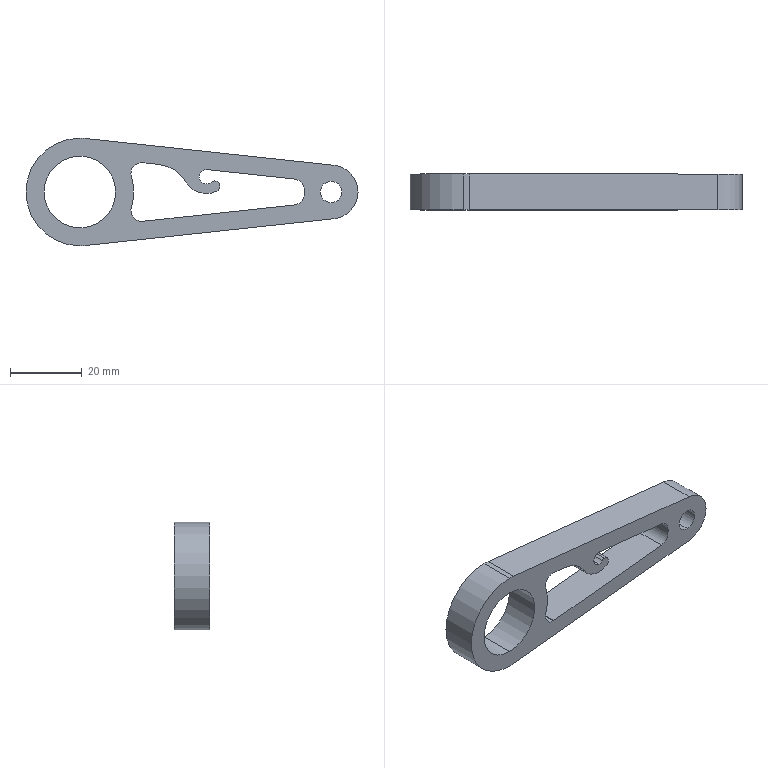Part | SolidWorks | features Fillet 3, ICE 2, Extrusion 1 | 1 solid | 29 faces | box 92.5 x 10 x 30 mm | volume 11719 mm3 | cylinder 22 | plane 7 | commonest cylinder face diameters 6 x7 30 x4 4 x3 20 x3 3 x2 15 x2
STEP:
#1=CARTESIAN_POINT('',(36.559,0.,2.727));
#2=VERTEX_POINT('',#1);
#3=CARTESIAN_POINT('',(37.534,0.,3.088));
#4=VERTEX_POINT('',#3);
#5=CARTESIAN_POINT('',(37.534,0.,1.588));
#6=DIRECTION('',(0.,1.,0.));
#7=DIRECTION('',(0.,0.,1.));
#8=AXIS2_PLACEMENT_3D('',#5,#6,#7);
#9=CIRCLE('',#8,1.5);
#10=EDGE_CURVE('',#2,#4,#9,.T.);
#11=ORIENTED_EDGE('',*,*,#10,.T.);
#12=CARTESIAN_POINT('',(37.534,10.,3.088));
#13=VERTEX_POINT('',#12);
#14=CARTESIAN_POINT('',(37.534,0.,3.088));
#15=DIRECTION('',(0.,1.,0.));
#16=VECTOR('',#15,1000.);
#17=LINE('',#14,#16);
#18=EDGE_CURVE('',#4,#13,#17,.T.);
#19=ORIENTED_EDGE('',*,*,#18,.T.);
#20=CARTESIAN_POINT('',(36.559,10.,2.727));
#21=VERTEX_POINT('',#20);
#22=CARTESIAN_POINT('',(37.534,10.,1.588));
#23=DIRECTION('',(0.,1.,0.));
#24=DIRECTION('',(0.,0.,1.));
#25=AXIS2_PLACEMENT_3D('',#22,#23,#24);
#26=CIRCLE('',#25,1.5);
#27=EDGE_CURVE('',#21,#13,#26,.T.);
#28=ORIENTED_EDGE('',*,*,#27,.F.);
#29=CARTESIAN_POINT('',(36.559,0.,2.727));
#30=DIRECTION('',(0.,1.,0.));
#31=VECTOR('',#30,1000.);
#32=LINE('',#29,#31);
#33=EDGE_CURVE('',#2,#21,#32,.T.);
#34=ORIENTED_EDGE('',*,*,#33,.F.);
#35=EDGE_LOOP('',(#11,#19,#28,#34));
#36=FACE_OUTER_BOUND('',#35,.T.);
#37=CARTESIAN_POINT('',(37.534,0.,1.588));
#38=DIRECTION('',(0.,1.,0.));
#39=DIRECTION('',(0.,0.,1.));
#40=AXIS2_PLACEMENT_3D('',#37,#38,#39);
#41=CYLINDRICAL_SURFACE('',#40,1.5);
#42=ADVANCED_FACE('',(#36),#41,.T.);
#43=CARTESIAN_POINT('',(35.259,0.,6.247));
#44=VERTEX_POINT('',#43);
#45=CARTESIAN_POINT('',(35.259,0.,2.247));
#46=VERTEX_POINT('',#45);
#47=CARTESIAN_POINT('',(35.259,0.,4.247));
#48=DIRECTION('',(0.,-1.,0.));
#49=DIRECTION('',(0.,0.,1.));
#50=AXIS2_PLACEMENT_3D('',#47,#48,#49);
#51=CIRCLE('',#50,2.);
#52=EDGE_CURVE('',#44,#46,#51,.T.);
#53=ORIENTED_EDGE('',*,*,#52,.T.);
#54=CARTESIAN_POINT('',(35.259,10.,2.247));
#55=VERTEX_POINT('',#54);
#56=CARTESIAN_POINT('',(35.259,0.,2.247));
#57=DIRECTION('',(0.,1.,0.));
#58=VECTOR('',#57,1000.);
#59=LINE('',#56,#58);
#60=EDGE_CURVE('',#46,#55,#59,.T.);
#61=ORIENTED_EDGE('',*,*,#60,.T.);
#62=CARTESIAN_POINT('',(35.259,10.,6.247));
#63=VERTEX_POINT('',#62);
#64=CARTESIAN_POINT('',(35.259,10.,4.247));
#65=DIRECTION('',(0.,-1.,0.));
#66=DIRECTION('',(0.,0.,1.));
#67=AXIS2_PLACEMENT_3D('',#64,#65,#66);
#68=CIRCLE('',#67,2.);
#69=EDGE_CURVE('',#63,#55,#68,.T.);
#70=ORIENTED_EDGE('',*,*,#69,.F.);
#71=CARTESIAN_POINT('',(35.259,0.,6.247));
#72=DIRECTION('',(0.,1.,0.));
#73=VECTOR('',#72,1000.);
#74=LINE('',#71,#73);
#75=EDGE_CURVE('',#44,#63,#74,.T.);
#76=ORIENTED_EDGE('',*,*,#75,.F.);
#77=EDGE_LOOP('',(#53,#61,#70,#76));
#78=FACE_OUTER_BOUND('',#77,.T.);
#79=CARTESIAN_POINT('',(35.259,0.,4.247));
#80=DIRECTION('',(0.,1.,0.));
#81=DIRECTION('',(0.,0.,1.));
#82=AXIS2_PLACEMENT_3D('',#79,#80,#81);
#83=CYLINDRICAL_SURFACE('',#82,2.);
#84=ADVANCED_FACE('',(#78),#83,.F.);
#85=CARTESIAN_POINT('',(35.473,0.,6.235));
#86=VERTEX_POINT('',#85);
#87=CARTESIAN_POINT('',(35.259,0.,4.247));
#88=DIRECTION('',(0.,-1.,0.));
#89=DIRECTION('',(0.,0.,1.));
#90=AXIS2_PLACEMENT_3D('',#87,#88,#89);
#91=CIRCLE('',#90,2.);
#92=EDGE_CURVE('',#86,#44,#91,.T.);
#93=ORIENTED_EDGE('',*,*,#92,.T.);
#94=ORIENTED_EDGE('',*,*,#75,.T.);
#95=CARTESIAN_POINT('',(35.473,10.,6.235));
#96=VERTEX_POINT('',#95);
#97=CARTESIAN_POINT('',(35.259,10.,4.247));
#98=DIRECTION('',(0.,-1.,0.));
#99=DIRECTION('',(0.,0.,1.));
#100=AXIS2_PLACEMENT_3D('',#97,#98,#99);
#101=CIRCLE('',#100,2.);
#102=EDGE_CURVE('',#96,#63,#101,.T.);
#103=ORIENTED_EDGE('',*,*,#102,.F.);
#104=CARTESIAN_POINT('',(35.473,0.,6.235));
#105=DIRECTION('',(0.,1.,0.));
#106=VECTOR('',#105,1000.);
#107=LINE('',#104,#106);
#108=EDGE_CURVE('',#86,#96,#107,.T.);
#109=ORIENTED_EDGE('',*,*,#108,.F.);
#110=EDGE_LOOP('',(#93,#94,#103,#109));
#111=FACE_OUTER_BOUND('',#110,.T.);
#112=CARTESIAN_POINT('',(35.259,0.,4.247));
#113=DIRECTION('',(0.,1.,0.));
#114=DIRECTION('',(0.,0.,1.));
#115=AXIS2_PLACEMENT_3D('',#112,#113,#114);
#116=CYLINDRICAL_SURFACE('',#115,2.);
#117=ADVANCED_FACE('',(#111),#116,.F.);
#118=CARTESIAN_POINT('',(17.238,10.,-8.183));
#119=VERTEX_POINT('',#118);
#120=CARTESIAN_POINT('',(17.559,10.,-8.166));
#121=VERTEX_POINT('',#120);
#122=CARTESIAN_POINT('',(17.238,10.,-5.183));
#123=DIRECTION('',(0.,-1.,0.));
#124=DIRECTION('',(0.,0.,1.));
#125=AXIS2_PLACEMENT_3D('',#122,#123,#124);
#126=CIRCLE('',#125,3.);
#127=EDGE_CURVE('',#119,#121,#126,.T.);
#128=ORIENTED_EDGE('',*,*,#127,.F.);
#129=CARTESIAN_POINT('',(17.238,0.,-8.183));
#130=VERTEX_POINT('',#129);
#131=CARTESIAN_POINT('',(17.238,10.,-8.183));
#132=DIRECTION('',(0.,-1.,0.));
#133=VECTOR('',#132,1000.);
#134=LINE('',#131,#133);
#135=EDGE_CURVE('',#119,#130,#134,.T.);
#136=ORIENTED_EDGE('',*,*,#135,.T.);
#137=CARTESIAN_POINT('',(17.559,0.,-8.166));
#138=VERTEX_POINT('',#137);
#139=CARTESIAN_POINT('',(17.238,0.,-5.183));
#140=DIRECTION('',(0.,1.,0.));
#141=DIRECTION('',(0.,0.,1.));
#142=AXIS2_PLACEMENT_3D('',#139,#140,#141);
#143=CIRCLE('',#142,3.);
#144=EDGE_CURVE('',#138,#130,#143,.T.);
#145=ORIENTED_EDGE('',*,*,#144,.F.);
#146=CARTESIAN_POINT('',(17.559,0.,-8.166));
#147=DIRECTION('',(0.,-1.,0.));
#148=VECTOR('',#147,1000.);
#149=LINE('',#146,#148);
#150=EDGE_CURVE('',#121,#138,#149,.T.);
#151=ORIENTED_EDGE('',*,*,#150,.F.);
#152=EDGE_LOOP('',(#128,#136,#145,#151));
#153=FACE_OUTER_BOUND('',#152,.T.);
#154=CARTESIAN_POINT('',(17.238,10.,-5.183));
#155=DIRECTION('',(0.,-1.,0.));
#156=DIRECTION('',(0.,0.,-1.));
#157=AXIS2_PLACEMENT_3D('',#154,#155,#156);
#158=CYLINDRICAL_SURFACE('',#157,3.);
#159=ADVANCED_FACE('',(#153),#158,.F.);
#160=CARTESIAN_POINT('',(70.,10.,-3.));
#161=VERTEX_POINT('',#160);
#162=CARTESIAN_POINT('',(70.,10.,3.));
#163=VERTEX_POINT('',#162);
#164=CARTESIAN_POINT('',(70.,10.,0.));
#165=DIRECTION('',(0.,1.,0.));
#166=DIRECTION('',(0.,0.,1.));
#167=AXIS2_PLACEMENT_3D('',#164,#165,#166);
#168=CIRCLE('',#167,3.);
#169=EDGE_CURVE('',#161,#163,#168,.T.);
#170=ORIENTED_EDGE('',*,*,#169,.T.);
#171=CARTESIAN_POINT('',(70.,0.,3.));
#172=VERTEX_POINT('',#171);
#173=CARTESIAN_POINT('',(70.,10.,3.));
#174=DIRECTION('',(0.,-1.,0.));
#175=VECTOR('',#174,1000.);
#176=LINE('',#173,#175);
#177=EDGE_CURVE('',#163,#172,#176,.T.);
#178=ORIENTED_EDGE('',*,*,#177,.T.);
#179=CARTESIAN_POINT('',(70.,0.,-3.));
#180=VERTEX_POINT('',#179);
#181=CARTESIAN_POINT('',(70.,0.,0.));
#182=DIRECTION('',(0.,1.,0.));
#183=DIRECTION('',(0.,0.,1.));
#184=AXIS2_PLACEMENT_3D('',#181,#182,#183);
#185=CIRCLE('',#184,3.);
#186=EDGE_CURVE('',#180,#172,#185,.T.);
#187=ORIENTED_EDGE('',*,*,#186,.F.);
#188=CARTESIAN_POINT('',(70.,10.,-3.));
#189=DIRECTION('',(0.,-1.,0.));
#190=VECTOR('',#189,1000.);
#191=LINE('',#188,#190);
#192=EDGE_CURVE('',#161,#180,#191,.T.);
#193=ORIENTED_EDGE('',*,*,#192,.F.);
#194=EDGE_LOOP('',(#170,#178,#187,#193));
#195=FACE_OUTER_BOUND('',#194,.T.);
#196=CARTESIAN_POINT('',(70.,10.,0.));
#197=DIRECTION('',(0.,-1.,0.));
#198=DIRECTION('',(0.,0.,-1.));
#199=AXIS2_PLACEMENT_3D('',#196,#197,#198);
#200=CYLINDRICAL_SURFACE('',#199,3.);
#201=ADVANCED_FACE('',(#195),#200,.F.);
#202=CARTESIAN_POINT('',(0.,10.,-10.));
#203=VERTEX_POINT('',#202);
#204=CARTESIAN_POINT('',(0.,10.,10.));
#205=VERTEX_POINT('',#204);
#206=CARTESIAN_POINT('',(0.,10.,0.));
#207=DIRECTION('',(0.,1.,0.));
#208=DIRECTION('',(0.,0.,1.));
#209=AXIS2_PLACEMENT_3D('',#206,#207,#208);
#210=CIRCLE('',#209,10.);
#211=EDGE_CURVE('',#203,#205,#210,.T.);
#212=ORIENTED_EDGE('',*,*,#211,.T.);
#213=CARTESIAN_POINT('',(0.,0.,10.));
#214=VERTEX_POINT('',#213);
#215=CARTESIAN_POINT('',(0.,10.,10.));
#216=DIRECTION('',(0.,-1.,0.));
#217=VECTOR('',#216,1000.);
#218=LINE('',#215,#217);
#219=EDGE_CURVE('',#205,#214,#218,.T.);
#220=ORIENTED_EDGE('',*,*,#219,.T.);
#221=CARTESIAN_POINT('',(0.,0.,-10.));
#222=VERTEX_POINT('',#221);
#223=CARTESIAN_POINT('',(0.,0.,0.));
#224=DIRECTION('',(0.,1.,0.));
#225=DIRECTION('',(0.,0.,1.));
#226=AXIS2_PLACEMENT_3D('',#223,#224,#225);
#227=CIRCLE('',#226,10.);
#228=EDGE_CURVE('',#222,#214,#227,.T.);
#229=ORIENTED_EDGE('',*,*,#228,.F.);
#230=CARTESIAN_POINT('',(0.,10.,-10.));
#231=DIRECTION('',(0.,-1.,0.));
#232=VECTOR('',#231,1000.);
#233=LINE('',#230,#232);
#234=EDGE_CURVE('',#203,#222,#233,.T.);
#235=ORIENTED_EDGE('',*,*,#234,.F.);
#236=EDGE_LOOP('',(#212,#220,#229,#235));
#237=FACE_OUTER_BOUND('',#236,.T.);
#238=CARTESIAN_POINT('',(0.,10.,0.));
#239=DIRECTION('',(0.,-1.,0.));
#240=DIRECTION('',(0.,0.,-1.));
#241=AXIS2_PLACEMENT_3D('',#238,#239,#240);
#242=CYLINDRICAL_SURFACE('',#241,10.);
#243=ADVANCED_FACE('',(#237),#242,.F.);
#244=CARTESIAN_POINT('',(0.,10.,15.));
#245=VERTEX_POINT('',#244);
#246=CARTESIAN_POINT('',(1.607,10.,14.914));
#247=VERTEX_POINT('',#246);
#248=CARTESIAN_POINT('',(0.,10.,0.));
#249=DIRECTION('',(0.,1.,0.));
#250=DIRECTION('',(0.,0.,1.));
#251=AXIS2_PLACEMENT_3D('',#248,#249,#250);
#252=CIRCLE('',#251,15.);
#253=EDGE_CURVE('',#245,#247,#252,.T.);
#254=ORIENTED_EDGE('',*,*,#253,.F.);
#255=CARTESIAN_POINT('',(0.,0.,15.));
#256=VERTEX_POINT('',#255);
#257=CARTESIAN_POINT('',(0.,10.,15.));
#258=DIRECTION('',(0.,-1.,0.));
#259=VECTOR('',#258,1000.);
#260=LINE('',#257,#259);
#261=EDGE_CURVE('',#245,#256,#260,.T.);
#262=ORIENTED_EDGE('',*,*,#261,.T.);
#263=CARTESIAN_POINT('',(1.607,0.,14.914));
#264=VERTEX_POINT('',#263);
#265=CARTESIAN_POINT('',(0.,0.,0.));
#266=DIRECTION('',(0.,1.,0.));
#267=DIRECTION('',(0.,0.,1.));
#268=AXIS2_PLACEMENT_3D('',#265,#266,#267);
#269=CIRCLE('',#268,15.);
#270=EDGE_CURVE('',#256,#264,#269,.T.);
#271=ORIENTED_EDGE('',*,*,#270,.T.);
#272=CARTESIAN_POINT('',(1.607,10.,14.914));
#273=DIRECTION('',(0.,-1.,0.));
#274=VECTOR('',#273,1000.);
#275=LINE('',#272,#274);
#276=EDGE_CURVE('',#247,#264,#275,.T.);
#277=ORIENTED_EDGE('',*,*,#276,.F.);
#278=EDGE_LOOP('',(#254,#262,#271,#277));
#279=FACE_OUTER_BOUND('',#278,.T.);
#280=CARTESIAN_POINT('',(0.,10.,0.));
#281=DIRECTION('',(0.,-1.,0.));
#282=DIRECTION('',(0.,0.,-1.));
#283=AXIS2_PLACEMENT_3D('',#280,#281,#282);
#284=CYLINDRICAL_SURFACE('',#283,15.);
#285=ADVANCED_FACE('',(#279),#284,.T.);
#286=ORIENTED_EDGE('',*,*,#261,.F.);
#287=CARTESIAN_POINT('',(0.,10.,-15.));
#288=VERTEX_POINT('',#287);
#289=CARTESIAN_POINT('',(0.,10.,0.));
#290=DIRECTION('',(0.,1.,0.));
#291=DIRECTION('',(0.,0.,1.));
#292=AXIS2_PLACEMENT_3D('',#289,#290,#291);
#293=CIRCLE('',#292,15.);
#294=EDGE_CURVE('',#288,#245,#293,.T.);
#295=ORIENTED_EDGE('',*,*,#294,.F.);
#296=CARTESIAN_POINT('',(0.,0.,-15.));
#297=VERTEX_POINT('',#296);
#298=CARTESIAN_POINT('',(0.,10.,-15.));
#299=DIRECTION('',(0.,-1.,0.));
#300=VECTOR('',#299,1000.);
#301=LINE('',#298,#300);
#302=EDGE_CURVE('',#288,#297,#301,.T.);
#303=ORIENTED_EDGE('',*,*,#302,.T.);
#304=CARTESIAN_POINT('',(0.,0.,0.));
#305=DIRECTION('',(0.,1.,0.));
#306=DIRECTION('',(0.,0.,1.));
#307=AXIS2_PLACEMENT_3D('',#304,#305,#306);
#308=CIRCLE('',#307,15.);
#309=EDGE_CURVE('',#297,#256,#308,.T.);
#310=ORIENTED_EDGE('',*,*,#309,.T.);
#311=EDGE_LOOP('',(#286,#295,#303,#310));
#312=FACE_OUTER_BOUND('',#311,.T.);
#313=CARTESIAN_POINT('',(0.,10.,0.));
#314=DIRECTION('',(0.,-1.,0.));
#315=DIRECTION('',(0.,0.,-1.));
#316=AXIS2_PLACEMENT_3D('',#313,#314,#315);
#317=CYLINDRICAL_SURFACE('',#316,15.);
#318=ADVANCED_FACE('',(#312),#317,.T.);
#319=ORIENTED_EDGE('',*,*,#108,.T.);
#320=CARTESIAN_POINT('',(59.84,10.,3.609));
#321=VERTEX_POINT('',#320);
#322=CARTESIAN_POINT('',(12.187,10.,8.745));
#323=DIRECTION('',(0.9942,0.,-0.1071));
#324=VECTOR('',#323,1000.);
#325=LINE('',#322,#324);
#326=EDGE_CURVE('',#96,#321,#325,.T.);
#327=ORIENTED_EDGE('',*,*,#326,.T.);
#328=CARTESIAN_POINT('',(59.84,0.,3.609));
#329=VERTEX_POINT('',#328);
#330=CARTESIAN_POINT('',(59.84,0.,3.609));
#331=DIRECTION('',(0.,-1.,0.));
#332=VECTOR('',#331,1000.);
#333=LINE('',#330,#332);
#334=EDGE_CURVE('',#321,#329,#333,.T.);
#335=ORIENTED_EDGE('',*,*,#334,.T.);
#336=CARTESIAN_POINT('',(12.187,0.,8.745));
#337=DIRECTION('',(0.9942,0.,-0.1071));
#338=VECTOR('',#337,1000.);
#339=LINE('',#336,#338);
#340=EDGE_CURVE('',#86,#329,#339,.T.);
#341=ORIENTED_EDGE('',*,*,#340,.F.);
#342=EDGE_LOOP('',(#319,#327,#335,#341));
#343=FACE_OUTER_BOUND('',#342,.T.);
#344=CARTESIAN_POINT('',(12.187,10.,8.745));
#345=DIRECTION('',(-0.1071,0.,-0.9942));
#346=DIRECTION('',(-0.9942,0.,0.1071));
#347=AXIS2_PLACEMENT_3D('',#344,#345,#346);
#348=PLANE('',#347);
#349=ADVANCED_FACE('',(#343),#348,.T.);
#350=CARTESIAN_POINT('',(17.559,10.,8.166));
#351=VERTEX_POINT('',#350);
#352=CARTESIAN_POINT('',(21.972,10.,7.69));
#353=VERTEX_POINT('',#352);
#354=CARTESIAN_POINT('',(12.187,10.,8.745));
#355=DIRECTION('',(0.9942,0.,-0.1071));
#356=VECTOR('',#355,1000.);
#357=LINE('',#354,#356);
#358=EDGE_CURVE('',#351,#353,#357,.T.);
#359=ORIENTED_EDGE('',*,*,#358,.F.);
#360=CARTESIAN_POINT('',(14.365,10.,4.319));
#361=VERTEX_POINT('',#360);
#362=CARTESIAN_POINT('',(17.238,10.,5.183));
#363=DIRECTION('',(0.,-1.,0.));
#364=DIRECTION('',(0.,0.,1.));
#365=AXIS2_PLACEMENT_3D('',#362,#363,#364);
#366=CIRCLE('',#365,3.);
#367=EDGE_CURVE('',#351,#361,#366,.T.);
#368=ORIENTED_EDGE('',*,*,#367,.T.);
#369=CARTESIAN_POINT('',(14.365,10.,-4.319));
#370=VERTEX_POINT('',#369);
#371=CARTESIAN_POINT('',(0.,10.,0.));
#372=DIRECTION('',(0.,-1.,0.));
#373=DIRECTION('',(0.,0.,1.));
#374=AXIS2_PLACEMENT_3D('',#371,#372,#373);
#375=CIRCLE('',#374,15.);
#376=EDGE_CURVE('',#370,#361,#375,.T.);
#377=ORIENTED_EDGE('',*,*,#376,.F.);
#378=CARTESIAN_POINT('',(17.238,10.,-5.183));
#379=DIRECTION('',(0.,-1.,0.));
#380=DIRECTION('',(0.,0.,1.));
#381=AXIS2_PLACEMENT_3D('',#378,#379,#380);
#382=CIRCLE('',#381,3.);
#383=EDGE_CURVE('',#370,#119,#382,.T.);
#384=ORIENTED_EDGE('',*,*,#383,.T.);
#385=ORIENTED_EDGE('',*,*,#127,.T.);
#386=CARTESIAN_POINT('',(59.84,10.,-3.609));
#387=VERTEX_POINT('',#386);
#388=CARTESIAN_POINT('',(12.187,10.,-8.745));
#389=DIRECTION('',(-0.9942,0.,-0.1071));
#390=VECTOR('',#389,1000.);
#391=LINE('',#388,#390);
#392=EDGE_CURVE('',#387,#121,#391,.T.);
#393=ORIENTED_EDGE('',*,*,#392,.F.);
#394=CARTESIAN_POINT('',(62.513,10.,-0.4476));
#395=VERTEX_POINT('',#394);
#396=CARTESIAN_POINT('',(59.519,10.,-0.6266));
#397=DIRECTION('',(0.,-1.,0.));
#398=DIRECTION('',(0.,0.,1.));
#399=AXIS2_PLACEMENT_3D('',#396,#397,#398);
#400=CIRCLE('',#399,3.);
#401=EDGE_CURVE('',#387,#395,#400,.T.);
#402=ORIENTED_EDGE('',*,*,#401,.T.);
#403=CARTESIAN_POINT('',(62.513,10.,0.4476));
#404=VERTEX_POINT('',#403);
#405=CARTESIAN_POINT('',(70.,10.,0.));
#406=DIRECTION('',(0.,-1.,0.));
#407=DIRECTION('',(0.,0.,1.));
#408=AXIS2_PLACEMENT_3D('',#405,#406,#407);
#409=CIRCLE('',#408,7.5);
#410=EDGE_CURVE('',#404,#395,#409,.T.);
#411=ORIENTED_EDGE('',*,*,#410,.F.);
#412=CARTESIAN_POINT('',(59.519,10.,0.6266));
#413=DIRECTION('',(0.,-1.,0.));
#414=DIRECTION('',(0.,0.,1.));
#415=AXIS2_PLACEMENT_3D('',#412,#413,#414);
#416=CIRCLE('',#415,3.);
#417=EDGE_CURVE('',#404,#321,#416,.T.);
#418=ORIENTED_EDGE('',*,*,#417,.T.);
#419=ORIENTED_EDGE('',*,*,#326,.F.);
#420=ORIENTED_EDGE('',*,*,#102,.T.);
#421=ORIENTED_EDGE('',*,*,#69,.T.);
#422=CARTESIAN_POINT('',(35.259,10.,4.247));
#423=DIRECTION('',(0.,-1.,0.));
#424=DIRECTION('',(0.,0.,1.));
#425=AXIS2_PLACEMENT_3D('',#422,#423,#424);
#426=CIRCLE('',#425,2.);
#427=EDGE_CURVE('',#55,#21,#426,.T.);
#428=ORIENTED_EDGE('',*,*,#427,.T.);
#429=ORIENTED_EDGE('',*,*,#27,.T.);
#430=CARTESIAN_POINT('',(38.193,10.,0.2398));
#431=VERTEX_POINT('',#430);
#432=CARTESIAN_POINT('',(37.534,10.,1.588));
#433=DIRECTION('',(0.,1.,0.));
#434=DIRECTION('',(0.,0.,1.));
#435=AXIS2_PLACEMENT_3D('',#432,#433,#434);
#436=CIRCLE('',#435,1.5);
#437=EDGE_CURVE('',#13,#431,#436,.T.);
#438=ORIENTED_EDGE('',*,*,#437,.T.);
#439=CARTESIAN_POINT('',(29.506,10.,2.841));
#440=VERTEX_POINT('',#439);
#441=CARTESIAN_POINT('',(35.259,10.,6.247));
#442=DIRECTION('',(0.,1.,0.));
#443=DIRECTION('',(0.,0.,1.));
#444=AXIS2_PLACEMENT_3D('',#441,#442,#443);
#445=CIRCLE('',#444,6.685);
#446=EDGE_CURVE('',#431,#440,#445,.T.);
#447=ORIENTED_EDGE('',*,*,#446,.T.);
#448=CARTESIAN_POINT('',(20.9,10.,-2.252));
#449=DIRECTION('',(0.,-1.,0.));
#450=DIRECTION('',(0.,0.,1.));
#451=AXIS2_PLACEMENT_3D('',#448,#449,#450);
#452=CIRCLE('',#451,10.);
#453=EDGE_CURVE('',#440,#353,#452,.T.);
#454=ORIENTED_EDGE('',*,*,#453,.T.);
#455=EDGE_LOOP('',(#359,#368,#377,#384,#385,#393,#402,#411,#418,#419,#420,#421,#428,#429,#438,#447,#454));
#456=FACE_BOUND('',#455,.T.);
#457=ORIENTED_EDGE('',*,*,#211,.F.);
#458=CARTESIAN_POINT('',(0.,10.,0.));
#459=DIRECTION('',(0.,1.,0.));
#460=DIRECTION('',(0.,0.,1.));
#461=AXIS2_PLACEMENT_3D('',#458,#459,#460);
#462=CIRCLE('',#461,10.);
#463=EDGE_CURVE('',#205,#203,#462,.T.);
#464=ORIENTED_EDGE('',*,*,#463,.F.);
#465=EDGE_LOOP('',(#457,#464));
#466=FACE_BOUND('',#465,.T.);
#467=CARTESIAN_POINT('',(1.607,10.,-14.914));
#468=VERTEX_POINT('',#467);
#469=CARTESIAN_POINT('',(0.,10.,0.));
#470=DIRECTION('',(0.,1.,0.));
#471=DIRECTION('',(0.,0.,1.));
#472=AXIS2_PLACEMENT_3D('',#469,#470,#471);
#473=CIRCLE('',#472,15.);
#474=EDGE_CURVE('',#468,#288,#473,.T.);
#475=ORIENTED_EDGE('',*,*,#474,.T.);
#476=ORIENTED_EDGE('',*,*,#294,.T.);
#477=ORIENTED_EDGE('',*,*,#253,.T.);
#478=CARTESIAN_POINT('',(70.804,10.,7.457));
#479=VERTEX_POINT('',#478);
#480=CARTESIAN_POINT('',(1.607,10.,14.914));
#481=DIRECTION('',(0.9942,0.,-0.1071));
#482=VECTOR('',#481,1000.);
#483=LINE('',#480,#482);
#484=EDGE_CURVE('',#247,#479,#483,.T.);
#485=ORIENTED_EDGE('',*,*,#484,.T.);
#486=CARTESIAN_POINT('',(70.804,10.,-7.457));
#487=VERTEX_POINT('',#486);
#488=CARTESIAN_POINT('',(70.,10.,0.));
#489=DIRECTION('',(0.,1.,0.));
#490=DIRECTION('',(0.,0.,1.));
#491=AXIS2_PLACEMENT_3D('',#488,#489,#490);
#492=CIRCLE('',#491,7.5);
#493=EDGE_CURVE('',#479,#487,#492,.T.);
#494=ORIENTED_EDGE('',*,*,#493,.T.);
#495=CARTESIAN_POINT('',(1.607,10.,-14.914));
#496=DIRECTION('',(-0.9942,0.,-0.1071));
#497=VECTOR('',#496,1000.);
#498=LINE('',#495,#497);
#499=EDGE_CURVE('',#487,#468,#498,.T.);
#500=ORIENTED_EDGE('',*,*,#499,.T.);
#501=EDGE_LOOP('',(#475,#476,#477,#485,#494,#500));
#502=FACE_OUTER_BOUND('',#501,.T.);
#503=ORIENTED_EDGE('',*,*,#169,.F.);
#504=CARTESIAN_POINT('',(70.,10.,0.));
#505=DIRECTION('',(0.,1.,0.));
#506=DIRECTION('',(0.,0.,1.));
#507=AXIS2_PLACEMENT_3D('',#504,#505,#506);
#508=CIRCLE('',#507,3.);
#509=EDGE_CURVE('',#163,#161,#508,.T.);
#510=ORIENTED_EDGE('',*,*,#509,.F.);
#511=EDGE_LOOP('',(#503,#510));
#512=FACE_BOUND('',#511,.T.);
#513=CARTESIAN_POINT('',(0.,10.,0.));
#514=DIRECTION('',(0.,1.,0.));
#515=DIRECTION('',(0.,0.,1.));
#516=AXIS2_PLACEMENT_3D('',#513,#514,#515);
#517=PLANE('',#516);
#518=ADVANCED_FACE('',(#456,#466,#502,#512),#517,.T.);
#519=ORIENTED_EDGE('',*,*,#228,.T.);
#520=CARTESIAN_POINT('',(0.,0.,0.));
#521=DIRECTION('',(0.,1.,0.));
#522=DIRECTION('',(0.,0.,1.));
#523=AXIS2_PLACEMENT_3D('',#520,#521,#522);
#524=CIRCLE('',#523,10.);
#525=EDGE_CURVE('',#214,#222,#524,.T.);
#526=ORIENTED_EDGE('',*,*,#525,.T.);
#527=EDGE_LOOP('',(#519,#526));
#528=FACE_BOUND('',#527,.T.);
#529=CARTESIAN_POINT('',(1.607,0.,-14.914));
#530=VERTEX_POINT('',#529);
#531=CARTESIAN_POINT('',(0.,0.,0.));
#532=DIRECTION('',(0.,1.,0.));
#533=DIRECTION('',(0.,0.,1.));
#534=AXIS2_PLACEMENT_3D('',#531,#532,#533);
#535=CIRCLE('',#534,15.);
#536=EDGE_CURVE('',#530,#297,#535,.T.);
#537=ORIENTED_EDGE('',*,*,#536,.F.);
#538=CARTESIAN_POINT('',(70.804,0.,-7.457));
#539=VERTEX_POINT('',#538);
#540=CARTESIAN_POINT('',(1.607,0.,-14.914));
#541=DIRECTION('',(-0.9942,0.,-0.1071));
#542=VECTOR('',#541,1000.);
#543=LINE('',#540,#542);
#544=EDGE_CURVE('',#539,#530,#543,.T.);
#545=ORIENTED_EDGE('',*,*,#544,.F.);
#546=CARTESIAN_POINT('',(70.804,0.,7.457));
#547=VERTEX_POINT('',#546);
#548=CARTESIAN_POINT('',(70.,0.,0.));
#549=DIRECTION('',(0.,1.,0.));
#550=DIRECTION('',(0.,0.,1.));
#551=AXIS2_PLACEMENT_3D('',#548,#549,#550);
#552=CIRCLE('',#551,7.5);
#553=EDGE_CURVE('',#547,#539,#552,.T.);
#554=ORIENTED_EDGE('',*,*,#553,.F.);
#555=CARTESIAN_POINT('',(1.607,0.,14.914));
#556=DIRECTION('',(0.9942,0.,-0.1071));
#557=VECTOR('',#556,1000.);
#558=LINE('',#555,#557);
#559=EDGE_CURVE('',#264,#547,#558,.T.);
#560=ORIENTED_EDGE('',*,*,#559,.F.);
#561=ORIENTED_EDGE('',*,*,#270,.F.);
#562=ORIENTED_EDGE('',*,*,#309,.F.);
#563=EDGE_LOOP('',(#537,#545,#554,#560,#561,#562));
#564=FACE_OUTER_BOUND('',#563,.T.);
#565=CARTESIAN_POINT('',(59.84,0.,-3.609));
#566=VERTEX_POINT('',#565);
#567=CARTESIAN_POINT('',(12.187,0.,-8.745));
#568=DIRECTION('',(-0.9942,0.,-0.1071));
#569=VECTOR('',#568,1000.);
#570=LINE('',#567,#569);
#571=EDGE_CURVE('',#566,#138,#570,.T.);
#572=ORIENTED_EDGE('',*,*,#571,.T.);
#573=ORIENTED_EDGE('',*,*,#144,.T.);
#574=CARTESIAN_POINT('',(14.365,0.,-4.319));
#575=VERTEX_POINT('',#574);
#576=CARTESIAN_POINT('',(17.238,0.,-5.183));
#577=DIRECTION('',(0.,1.,0.));
#578=DIRECTION('',(0.,0.,1.));
#579=AXIS2_PLACEMENT_3D('',#576,#577,#578);
#580=CIRCLE('',#579,3.);
#581=EDGE_CURVE('',#130,#575,#580,.T.);
#582=ORIENTED_EDGE('',*,*,#581,.T.);
#583=CARTESIAN_POINT('',(14.365,0.,4.319));
#584=VERTEX_POINT('',#583);
#585=CARTESIAN_POINT('',(0.,0.,0.));
#586=DIRECTION('',(0.,-1.,0.));
#587=DIRECTION('',(0.,0.,1.));
#588=AXIS2_PLACEMENT_3D('',#585,#586,#587);
#589=CIRCLE('',#588,15.);
#590=EDGE_CURVE('',#575,#584,#589,.T.);
#591=ORIENTED_EDGE('',*,*,#590,.T.);
#592=CARTESIAN_POINT('',(17.559,0.,8.166));
#593=VERTEX_POINT('',#592);
#594=CARTESIAN_POINT('',(17.238,0.,5.183));
#595=DIRECTION('',(0.,1.,0.));
#596=DIRECTION('',(0.,0.,1.));
#597=AXIS2_PLACEMENT_3D('',#594,#595,#596);
#598=CIRCLE('',#597,3.);
#599=EDGE_CURVE('',#584,#593,#598,.T.);
#600=ORIENTED_EDGE('',*,*,#599,.T.);
#601=CARTESIAN_POINT('',(21.972,0.,7.69));
#602=VERTEX_POINT('',#601);
#603=CARTESIAN_POINT('',(12.187,0.,8.745));
#604=DIRECTION('',(0.9942,0.,-0.1071));
#605=VECTOR('',#604,1000.);
#606=LINE('',#603,#605);
#607=EDGE_CURVE('',#593,#602,#606,.T.);
#608=ORIENTED_EDGE('',*,*,#607,.T.);
#609=CARTESIAN_POINT('',(29.506,0.,2.841));
#610=VERTEX_POINT('',#609);
#611=CARTESIAN_POINT('',(20.9,0.,-2.252));
#612=DIRECTION('',(0.,1.,0.));
#613=DIRECTION('',(0.,0.,1.));
#614=AXIS2_PLACEMENT_3D('',#611,#612,#613);
#615=CIRCLE('',#614,10.);
#616=EDGE_CURVE('',#602,#610,#615,.T.);
#617=ORIENTED_EDGE('',*,*,#616,.T.);
#618=CARTESIAN_POINT('',(38.193,0.,0.2398));
#619=VERTEX_POINT('',#618);
#620=CARTESIAN_POINT('',(35.259,0.,6.247));
#621=DIRECTION('',(0.,1.,0.));
#622=DIRECTION('',(0.,0.,1.));
#623=AXIS2_PLACEMENT_3D('',#620,#621,#622);
#624=CIRCLE('',#623,6.685);
#625=EDGE_CURVE('',#619,#610,#624,.T.);
#626=ORIENTED_EDGE('',*,*,#625,.F.);
#627=CARTESIAN_POINT('',(37.534,0.,1.588));
#628=DIRECTION('',(0.,1.,0.));
#629=DIRECTION('',(0.,0.,1.));
#630=AXIS2_PLACEMENT_3D('',#627,#628,#629);
#631=CIRCLE('',#630,1.5);
#632=EDGE_CURVE('',#4,#619,#631,.T.);
#633=ORIENTED_EDGE('',*,*,#632,.F.);
#634=ORIENTED_EDGE('',*,*,#10,.F.);
#635=CARTESIAN_POINT('',(35.259,0.,4.247));
#636=DIRECTION('',(0.,-1.,0.));
#637=DIRECTION('',(0.,0.,1.));
#638=AXIS2_PLACEMENT_3D('',#635,#636,#637);
#639=CIRCLE('',#638,2.);
#640=EDGE_CURVE('',#46,#2,#639,.T.);
#641=ORIENTED_EDGE('',*,*,#640,.F.);
#642=ORIENTED_EDGE('',*,*,#52,.F.);
#643=ORIENTED_EDGE('',*,*,#92,.F.);
#644=ORIENTED_EDGE('',*,*,#340,.T.);
#645=CARTESIAN_POINT('',(62.513,0.,0.4476));
#646=VERTEX_POINT('',#645);
#647=CARTESIAN_POINT('',(59.519,0.,0.6266));
#648=DIRECTION('',(0.,1.,0.));
#649=DIRECTION('',(0.,0.,1.));
#650=AXIS2_PLACEMENT_3D('',#647,#648,#649);
#651=CIRCLE('',#650,3.);
#652=EDGE_CURVE('',#329,#646,#651,.T.);
#653=ORIENTED_EDGE('',*,*,#652,.T.);
#654=CARTESIAN_POINT('',(62.513,0.,-0.4476));
#655=VERTEX_POINT('',#654);
#656=CARTESIAN_POINT('',(70.,0.,0.));
#657=DIRECTION('',(0.,-1.,0.));
#658=DIRECTION('',(0.,0.,1.));
#659=AXIS2_PLACEMENT_3D('',#656,#657,#658);
#660=CIRCLE('',#659,7.5);
#661=EDGE_CURVE('',#646,#655,#660,.T.);
#662=ORIENTED_EDGE('',*,*,#661,.T.);
#663=CARTESIAN_POINT('',(59.519,0.,-0.6266));
#664=DIRECTION('',(0.,1.,0.));
#665=DIRECTION('',(0.,0.,1.));
#666=AXIS2_PLACEMENT_3D('',#663,#664,#665);
#667=CIRCLE('',#666,3.);
#668=EDGE_CURVE('',#655,#566,#667,.T.);
#669=ORIENTED_EDGE('',*,*,#668,.T.);
#670=EDGE_LOOP('',(#572,#573,#582,#591,#600,#608,#617,#626,#633,#634,#641,#642,#643,#644,#653,#662,#669));
#671=FACE_BOUND('',#670,.T.);
#672=ORIENTED_EDGE('',*,*,#186,.T.);
#673=CARTESIAN_POINT('',(70.,0.,0.));
#674=DIRECTION('',(0.,1.,0.));
#675=DIRECTION('',(0.,0.,1.));
#676=AXIS2_PLACEMENT_3D('',#673,#674,#675);
#677=CIRCLE('',#676,3.);
#678=EDGE_CURVE('',#172,#180,#677,.T.);
#679=ORIENTED_EDGE('',*,*,#678,.T.);
#680=EDGE_LOOP('',(#672,#679));
#681=FACE_BOUND('',#680,.T.);
#682=CARTESIAN_POINT('',(0.,0.,0.));
#683=DIRECTION('',(0.,1.,0.));
#684=DIRECTION('',(0.,0.,1.));
#685=AXIS2_PLACEMENT_3D('',#682,#683,#684);
#686=PLANE('',#685);
#687=ADVANCED_FACE('',(#528,#564,#671,#681),#686,.F.);
#688=ORIENTED_EDGE('',*,*,#302,.F.);
#689=ORIENTED_EDGE('',*,*,#474,.F.);
#690=CARTESIAN_POINT('',(1.607,10.,-14.914));
#691=DIRECTION('',(0.,-1.,0.));
#692=VECTOR('',#691,1000.);
#693=LINE('',#690,#692);
#694=EDGE_CURVE('',#468,#530,#693,.T.);
#695=ORIENTED_EDGE('',*,*,#694,.T.);
#696=ORIENTED_EDGE('',*,*,#536,.T.);
#697=EDGE_LOOP('',(#688,#689,#695,#696));
#698=FACE_OUTER_BOUND('',#697,.T.);
#699=CARTESIAN_POINT('',(0.,10.,0.));
#700=DIRECTION('',(0.,-1.,0.));
#701=DIRECTION('',(0.,0.,-1.));
#702=AXIS2_PLACEMENT_3D('',#699,#700,#701);
#703=CYLINDRICAL_SURFACE('',#702,15.);
#704=ADVANCED_FACE('',(#698),#703,.T.);
#705=ORIENTED_EDGE('',*,*,#559,.T.);
#706=CARTESIAN_POINT('',(70.804,10.,7.457));
#707=DIRECTION('',(0.,-1.,0.));
#708=VECTOR('',#707,1000.);
#709=LINE('',#706,#708);
#710=EDGE_CURVE('',#479,#547,#709,.T.);
#711=ORIENTED_EDGE('',*,*,#710,.F.);
#712=ORIENTED_EDGE('',*,*,#484,.F.);
#713=ORIENTED_EDGE('',*,*,#276,.T.);
#714=EDGE_LOOP('',(#705,#711,#712,#713));
#715=FACE_OUTER_BOUND('',#714,.T.);
#716=CARTESIAN_POINT('',(1.607,10.,14.914));
#717=DIRECTION('',(-0.1071,0.,-0.9942));
#718=DIRECTION('',(-0.9942,0.,0.1071));
#719=AXIS2_PLACEMENT_3D('',#716,#717,#718);
#720=PLANE('',#719);
#721=ADVANCED_FACE('',(#715),#720,.F.);
#722=ORIENTED_EDGE('',*,*,#553,.T.);
#723=CARTESIAN_POINT('',(70.804,10.,-7.457));
#724=DIRECTION('',(0.,-1.,0.));
#725=VECTOR('',#724,1000.);
#726=LINE('',#723,#725);
#727=EDGE_CURVE('',#487,#539,#726,.T.);
#728=ORIENTED_EDGE('',*,*,#727,.F.);
#729=ORIENTED_EDGE('',*,*,#493,.F.);
#730=ORIENTED_EDGE('',*,*,#710,.T.);
#731=EDGE_LOOP('',(#722,#728,#729,#730));
#732=FACE_OUTER_BOUND('',#731,.T.);
#733=CARTESIAN_POINT('',(70.,10.,0.));
#734=DIRECTION('',(0.,-1.,0.));
#735=DIRECTION('',(0.,0.,-1.));
#736=AXIS2_PLACEMENT_3D('',#733,#734,#735);
#737=CYLINDRICAL_SURFACE('',#736,7.5);
#738=ADVANCED_FACE('',(#732),#737,.T.);
#739=ORIENTED_EDGE('',*,*,#544,.T.);
#740=ORIENTED_EDGE('',*,*,#694,.F.);
#741=ORIENTED_EDGE('',*,*,#499,.F.);
#742=ORIENTED_EDGE('',*,*,#727,.T.);
#743=EDGE_LOOP('',(#739,#740,#741,#742));
#744=FACE_OUTER_BOUND('',#743,.T.);
#745=CARTESIAN_POINT('',(1.607,10.,-14.914));
#746=DIRECTION('',(-0.1071,0.,0.9942));
#747=DIRECTION('',(0.9942,0.,0.1071));
#748=AXIS2_PLACEMENT_3D('',#745,#746,#747);
#749=PLANE('',#748);
#750=ADVANCED_FACE('',(#744),#749,.F.);
#751=ORIENTED_EDGE('',*,*,#219,.F.);
#752=ORIENTED_EDGE('',*,*,#463,.T.);
#753=ORIENTED_EDGE('',*,*,#234,.T.);
#754=ORIENTED_EDGE('',*,*,#525,.F.);
#755=EDGE_LOOP('',(#751,#752,#753,#754));
#756=FACE_OUTER_BOUND('',#755,.T.);
#757=CARTESIAN_POINT('',(0.,10.,0.));
#758=DIRECTION('',(0.,-1.,0.));
#759=DIRECTION('',(0.,0.,-1.));
#760=AXIS2_PLACEMENT_3D('',#757,#758,#759);
#761=CYLINDRICAL_SURFACE('',#760,10.);
#762=ADVANCED_FACE('',(#756),#761,.F.);
#763=ORIENTED_EDGE('',*,*,#376,.T.);
#764=CARTESIAN_POINT('',(14.365,10.,4.319));
#765=DIRECTION('',(0.,-1.,0.));
#766=VECTOR('',#765,1000.);
#767=LINE('',#764,#766);
#768=EDGE_CURVE('',#361,#584,#767,.T.);
#769=ORIENTED_EDGE('',*,*,#768,.T.);
#770=ORIENTED_EDGE('',*,*,#590,.F.);
#771=CARTESIAN_POINT('',(14.365,10.,-4.319));
#772=DIRECTION('',(0.,1.,0.));
#773=VECTOR('',#772,1000.);
#774=LINE('',#771,#773);
#775=EDGE_CURVE('',#575,#370,#774,.T.);
#776=ORIENTED_EDGE('',*,*,#775,.T.);
#777=EDGE_LOOP('',(#763,#769,#770,#776));
#778=FACE_OUTER_BOUND('',#777,.T.);
#779=CARTESIAN_POINT('',(0.,10.,0.));
#780=DIRECTION('',(0.,-1.,0.));
#781=DIRECTION('',(0.,0.,-1.));
#782=AXIS2_PLACEMENT_3D('',#779,#780,#781);
#783=CYLINDRICAL_SURFACE('',#782,15.);
#784=ADVANCED_FACE('',(#778),#783,.T.);
#785=ORIENTED_EDGE('',*,*,#358,.T.);
#786=CARTESIAN_POINT('',(21.972,0.,7.69));
#787=DIRECTION('',(0.,-1.,0.));
#788=VECTOR('',#787,1000.);
#789=LINE('',#786,#788);
#790=EDGE_CURVE('',#353,#602,#789,.T.);
#791=ORIENTED_EDGE('',*,*,#790,.T.);
#792=ORIENTED_EDGE('',*,*,#607,.F.);
#793=CARTESIAN_POINT('',(17.559,10.,8.166));
#794=DIRECTION('',(0.,1.,0.));
#795=VECTOR('',#794,1000.);
#796=LINE('',#793,#795);
#797=EDGE_CURVE('',#593,#351,#796,.T.);
#798=ORIENTED_EDGE('',*,*,#797,.T.);
#799=EDGE_LOOP('',(#785,#791,#792,#798));
#800=FACE_OUTER_BOUND('',#799,.T.);
#801=CARTESIAN_POINT('',(12.187,10.,8.745));
#802=DIRECTION('',(-0.1071,0.,-0.9942));
#803=DIRECTION('',(-0.9942,0.,0.1071));
#804=AXIS2_PLACEMENT_3D('',#801,#802,#803);
#805=PLANE('',#804);
#806=ADVANCED_FACE('',(#800),#805,.T.);
#807=ORIENTED_EDGE('',*,*,#661,.F.);
#808=CARTESIAN_POINT('',(62.513,10.,0.4476));
#809=DIRECTION('',(0.,1.,0.));
#810=VECTOR('',#809,1000.);
#811=LINE('',#808,#810);
#812=EDGE_CURVE('',#646,#404,#811,.T.);
#813=ORIENTED_EDGE('',*,*,#812,.T.);
#814=ORIENTED_EDGE('',*,*,#410,.T.);
#815=CARTESIAN_POINT('',(62.513,10.,-0.4476));
#816=DIRECTION('',(0.,-1.,0.));
#817=VECTOR('',#816,1000.);
#818=LINE('',#815,#817);
#819=EDGE_CURVE('',#395,#655,#818,.T.);
#820=ORIENTED_EDGE('',*,*,#819,.T.);
#821=EDGE_LOOP('',(#807,#813,#814,#820));
#822=FACE_OUTER_BOUND('',#821,.T.);
#823=CARTESIAN_POINT('',(70.,10.,0.));
#824=DIRECTION('',(0.,-1.,0.));
#825=DIRECTION('',(0.,0.,-1.));
#826=AXIS2_PLACEMENT_3D('',#823,#824,#825);
#827=CYLINDRICAL_SURFACE('',#826,7.5);
#828=ADVANCED_FACE('',(#822),#827,.T.);
#829=ORIENTED_EDGE('',*,*,#571,.F.);
#830=CARTESIAN_POINT('',(59.84,10.,-3.609));
#831=DIRECTION('',(0.,1.,0.));
#832=VECTOR('',#831,1000.);
#833=LINE('',#830,#832);
#834=EDGE_CURVE('',#566,#387,#833,.T.);
#835=ORIENTED_EDGE('',*,*,#834,.T.);
#836=ORIENTED_EDGE('',*,*,#392,.T.);
#837=ORIENTED_EDGE('',*,*,#150,.T.);
#838=EDGE_LOOP('',(#829,#835,#836,#837));
#839=FACE_OUTER_BOUND('',#838,.T.);
#840=CARTESIAN_POINT('',(12.187,10.,-8.745));
#841=DIRECTION('',(-0.1071,0.,0.9942));
#842=DIRECTION('',(0.9942,0.,0.1071));
#843=AXIS2_PLACEMENT_3D('',#840,#841,#842);
#844=PLANE('',#843);
#845=ADVANCED_FACE('',(#839),#844,.T.);
#846=ORIENTED_EDGE('',*,*,#177,.F.);
#847=ORIENTED_EDGE('',*,*,#509,.T.);
#848=ORIENTED_EDGE('',*,*,#192,.T.);
#849=ORIENTED_EDGE('',*,*,#678,.F.);
#850=EDGE_LOOP('',(#846,#847,#848,#849));
#851=FACE_OUTER_BOUND('',#850,.T.);
#852=CARTESIAN_POINT('',(70.,10.,0.));
#853=DIRECTION('',(0.,-1.,0.));
#854=DIRECTION('',(0.,0.,-1.));
#855=AXIS2_PLACEMENT_3D('',#852,#853,#854);
#856=CYLINDRICAL_SURFACE('',#855,3.);
#857=ADVANCED_FACE('',(#851),#856,.F.);
#858=ORIENTED_EDGE('',*,*,#417,.F.);
#859=ORIENTED_EDGE('',*,*,#812,.F.);
#860=ORIENTED_EDGE('',*,*,#652,.F.);
#861=ORIENTED_EDGE('',*,*,#334,.F.);
#862=EDGE_LOOP('',(#858,#859,#860,#861));
#863=FACE_OUTER_BOUND('',#862,.T.);
#864=CARTESIAN_POINT('',(59.519,10.,0.6266));
#865=DIRECTION('',(0.,-1.,0.));
#866=DIRECTION('',(0.,0.,-1.));
#867=AXIS2_PLACEMENT_3D('',#864,#865,#866);
#868=CYLINDRICAL_SURFACE('',#867,3.);
#869=ADVANCED_FACE('',(#863),#868,.F.);
#870=ORIENTED_EDGE('',*,*,#401,.F.);
#871=ORIENTED_EDGE('',*,*,#834,.F.);
#872=ORIENTED_EDGE('',*,*,#668,.F.);
#873=ORIENTED_EDGE('',*,*,#819,.F.);
#874=EDGE_LOOP('',(#870,#871,#872,#873));
#875=FACE_OUTER_BOUND('',#874,.T.);
#876=CARTESIAN_POINT('',(59.519,10.,-0.6266));
#877=DIRECTION('',(0.,-1.,0.));
#878=DIRECTION('',(0.,0.,-1.));
#879=AXIS2_PLACEMENT_3D('',#876,#877,#878);
#880=CYLINDRICAL_SURFACE('',#879,3.);
#881=ADVANCED_FACE('',(#875),#880,.F.);
#882=ORIENTED_EDGE('',*,*,#367,.F.);
#883=ORIENTED_EDGE('',*,*,#797,.F.);
#884=ORIENTED_EDGE('',*,*,#599,.F.);
#885=ORIENTED_EDGE('',*,*,#768,.F.);
#886=EDGE_LOOP('',(#882,#883,#884,#885));
#887=FACE_OUTER_BOUND('',#886,.T.);
#888=CARTESIAN_POINT('',(17.238,10.,5.183));
#889=DIRECTION('',(0.,-1.,0.));
#890=DIRECTION('',(0.,0.,-1.));
#891=AXIS2_PLACEMENT_3D('',#888,#889,#890);
#892=CYLINDRICAL_SURFACE('',#891,3.);
#893=ADVANCED_FACE('',(#887),#892,.F.);
#894=ORIENTED_EDGE('',*,*,#135,.F.);
#895=ORIENTED_EDGE('',*,*,#383,.F.);
#896=ORIENTED_EDGE('',*,*,#775,.F.);
#897=ORIENTED_EDGE('',*,*,#581,.F.);
#898=EDGE_LOOP('',(#894,#895,#896,#897));
#899=FACE_OUTER_BOUND('',#898,.T.);
#900=CARTESIAN_POINT('',(17.238,10.,-5.183));
#901=DIRECTION('',(0.,-1.,0.));
#902=DIRECTION('',(0.,0.,-1.));
#903=AXIS2_PLACEMENT_3D('',#900,#901,#902);
#904=CYLINDRICAL_SURFACE('',#903,3.);
#905=ADVANCED_FACE('',(#899),#904,.F.);
#906=ORIENTED_EDGE('',*,*,#60,.F.);
#907=ORIENTED_EDGE('',*,*,#640,.T.);
#908=ORIENTED_EDGE('',*,*,#33,.T.);
#909=ORIENTED_EDGE('',*,*,#427,.F.);
#910=EDGE_LOOP('',(#906,#907,#908,#909));
#911=FACE_OUTER_BOUND('',#910,.T.);
#912=CARTESIAN_POINT('',(35.259,0.,4.247));
#913=DIRECTION('',(0.,1.,0.));
#914=DIRECTION('',(0.,0.,1.));
#915=AXIS2_PLACEMENT_3D('',#912,#913,#914);
#916=CYLINDRICAL_SURFACE('',#915,2.);
#917=ADVANCED_FACE('',(#911),#916,.F.);
#918=ORIENTED_EDGE('',*,*,#625,.T.);
#919=CARTESIAN_POINT('',(29.506,0.,2.841));
#920=DIRECTION('',(0.,1.,0.));
#921=VECTOR('',#920,1000.);
#922=LINE('',#919,#921);
#923=EDGE_CURVE('',#610,#440,#922,.T.);
#924=ORIENTED_EDGE('',*,*,#923,.T.);
#925=ORIENTED_EDGE('',*,*,#446,.F.);
#926=CARTESIAN_POINT('',(38.193,0.,0.2398));
#927=DIRECTION('',(0.,1.,0.));
#928=VECTOR('',#927,1000.);
#929=LINE('',#926,#928);
#930=EDGE_CURVE('',#619,#431,#929,.T.);
#931=ORIENTED_EDGE('',*,*,#930,.F.);
#932=EDGE_LOOP('',(#918,#924,#925,#931));
#933=FACE_OUTER_BOUND('',#932,.T.);
#934=CARTESIAN_POINT('',(35.259,0.,6.247));
#935=DIRECTION('',(0.,1.,0.));
#936=DIRECTION('',(0.,0.,1.));
#937=AXIS2_PLACEMENT_3D('',#934,#935,#936);
#938=CYLINDRICAL_SURFACE('',#937,6.685);
#939=ADVANCED_FACE('',(#933),#938,.T.);
#940=ORIENTED_EDGE('',*,*,#18,.F.);
#941=ORIENTED_EDGE('',*,*,#632,.T.);
#942=ORIENTED_EDGE('',*,*,#930,.T.);
#943=ORIENTED_EDGE('',*,*,#437,.F.);
#944=EDGE_LOOP('',(#940,#941,#942,#943));
#945=FACE_OUTER_BOUND('',#944,.T.);
#946=CARTESIAN_POINT('',(37.534,0.,1.588));
#947=DIRECTION('',(0.,1.,0.));
#948=DIRECTION('',(0.,0.,1.));
#949=AXIS2_PLACEMENT_3D('',#946,#947,#948);
#950=CYLINDRICAL_SURFACE('',#949,1.5);
#951=ADVANCED_FACE('',(#945),#950,.T.);
#952=ORIENTED_EDGE('',*,*,#616,.F.);
#953=ORIENTED_EDGE('',*,*,#790,.F.);
#954=ORIENTED_EDGE('',*,*,#453,.F.);
#955=ORIENTED_EDGE('',*,*,#923,.F.);
#956=EDGE_LOOP('',(#952,#953,#954,#955));
#957=FACE_OUTER_BOUND('',#956,.T.);
#958=CARTESIAN_POINT('',(20.9,0.,-2.252));
#959=DIRECTION('',(0.,1.,0.));
#960=DIRECTION('',(0.,0.,1.));
#961=AXIS2_PLACEMENT_3D('',#958,#959,#960);
#962=CYLINDRICAL_SURFACE('',#961,10.);
#963=ADVANCED_FACE('',(#957),#962,.F.);
#964=CLOSED_SHELL('',(#42,#84,#117,#159,#201,#243,#285,#318,#349,#518,#687,#704,#721,#738,#750,#762,#784,#806,#828,#845,#857,#869,#881,#893,#905,#917,#939,#951,#963));
#965=MANIFOLD_SOLID_BREP('',#964);
#966=CARTESIAN_POINT('',(0.,0.,0.));
#967=DIRECTION('',(0.,0.,1.));
#968=DIRECTION('',(1.,0.,0.));
#969=AXIS2_PLACEMENT_3D('',#966,#967,#968);
#970=(LENGTH_UNIT()NAMED_UNIT(*)SI_UNIT(.MILLI.,.METRE.));
#971=UNCERTAINTY_MEASURE_WITH_UNIT(LENGTH_MEASURE(0.00001),#970,'','');
#972=(NAMED_UNIT(*)PLANE_ANGLE_UNIT()SI_UNIT($,.RADIAN.));
#973=(NAMED_UNIT(*)SI_UNIT($,.STERADIAN.)SOLID_ANGLE_UNIT());
#974=(GEOMETRIC_REPRESENTATION_CONTEXT(3)GLOBAL_UNCERTAINTY_ASSIGNED_CONTEXT((#971))GLOBAL_UNIT_ASSIGNED_CONTEXT((#970,#972,#973))REPRESENTATION_CONTEXT('',''));
#975=ADVANCED_BREP_SHAPE_REPRESENTATION('',(#965,#969),#974);